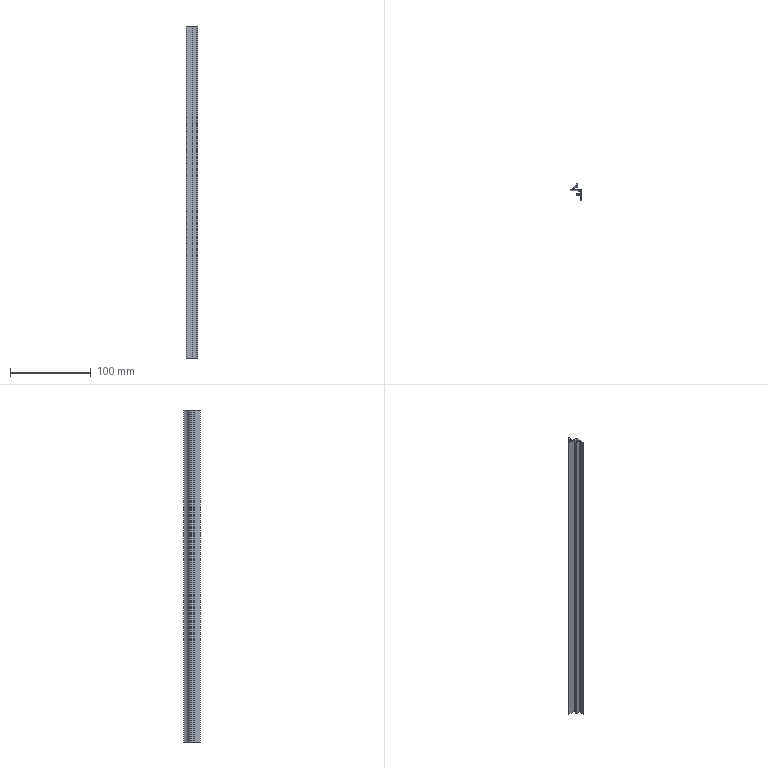Part | SolidWorks | features BaseBody 1, ICE 1, MoveFace 1 | 1 solid | 27 faces | box 14 x 20.3 x 410 mm | volume 20875 mm3 | plane 20 | cylinder 7 | commonest cylinder face diameters 0.387 x2 0.8 x2 0.4 x1 20 x1 22 x1
STEP:
#1=CARTESIAN_POINT('',(-5.304,-0.625,200.));
#2=VERTEX_POINT('',#1);
#3=CARTESIAN_POINT('',(-5.449,-0.8125,200.));
#4=VERTEX_POINT('',#3);
#5=CARTESIAN_POINT('',(-5.255,-0.8125,200.));
#6=DIRECTION('',(0.,0.,1.));
#7=DIRECTION('',(-1.,0.,0.));
#8=AXIS2_PLACEMENT_3D('',#5,#6,#7);
#9=CIRCLE('',#8,0.1937);
#10=EDGE_CURVE('',#2,#4,#9,.T.);
#11=ORIENTED_EDGE('',*,*,#10,.T.);
#12=CARTESIAN_POINT('',(-5.449,-0.8125,-210.));
#13=VERTEX_POINT('',#12);
#14=CARTESIAN_POINT('',(-5.449,-0.8125,230.));
#15=DIRECTION('',(0.,0.,-1.));
#16=VECTOR('',#15,1000.);
#17=LINE('',#14,#16);
#18=EDGE_CURVE('',#4,#13,#17,.T.);
#19=ORIENTED_EDGE('',*,*,#18,.T.);
#20=CARTESIAN_POINT('',(-5.304,-0.625,-210.));
#21=VERTEX_POINT('',#20);
#22=CARTESIAN_POINT('',(-5.255,-0.8125,-210.));
#23=DIRECTION('',(0.,0.,-1.));
#24=DIRECTION('',(1.,0.,0.));
#25=AXIS2_PLACEMENT_3D('',#22,#23,#24);
#26=CIRCLE('',#25,0.1937);
#27=EDGE_CURVE('',#13,#21,#26,.T.);
#28=ORIENTED_EDGE('',*,*,#27,.T.);
#29=CARTESIAN_POINT('',(-5.304,-0.625,230.));
#30=DIRECTION('',(0.,0.,-1.));
#31=VECTOR('',#30,1000.);
#32=LINE('',#29,#31);
#33=EDGE_CURVE('',#2,#21,#32,.T.);
#34=ORIENTED_EDGE('',*,*,#33,.F.);
#35=EDGE_LOOP('',(#11,#19,#28,#34));
#36=FACE_OUTER_BOUND('',#35,.T.);
#37=CARTESIAN_POINT('',(-5.255,-0.8125,230.));
#38=DIRECTION('',(0.,0.,-1.));
#39=DIRECTION('',(-1.,0.,0.));
#40=AXIS2_PLACEMENT_3D('',#37,#38,#39);
#41=CYLINDRICAL_SURFACE('',#40,0.1937);
#42=ADVANCED_FACE('',(#36),#41,.F.);
#43=CARTESIAN_POINT('',(5.,-1.,-210.));
#44=VERTEX_POINT('',#43);
#45=CARTESIAN_POINT('',(5.,-14.3,-210.));
#46=VERTEX_POINT('',#45);
#47=CARTESIAN_POINT('',(5.,29.623,-210.));
#48=DIRECTION('',(0.,-1.,0.));
#49=VECTOR('',#48,1000.);
#50=LINE('',#47,#49);
#51=EDGE_CURVE('',#44,#46,#50,.T.);
#52=ORIENTED_EDGE('',*,*,#51,.F.);
#53=CARTESIAN_POINT('',(5.,-1.,200.));
#54=VERTEX_POINT('',#53);
#55=CARTESIAN_POINT('',(5.,-1.,230.));
#56=DIRECTION('',(0.,0.,-1.));
#57=VECTOR('',#56,1000.);
#58=LINE('',#55,#57);
#59=EDGE_CURVE('',#54,#44,#58,.T.);
#60=ORIENTED_EDGE('',*,*,#59,.F.);
#61=CARTESIAN_POINT('',(5.,-14.3,200.));
#62=VERTEX_POINT('',#61);
#63=CARTESIAN_POINT('',(5.,-14.3,200.));
#64=DIRECTION('',(0.,1.,0.));
#65=VECTOR('',#64,1000.);
#66=LINE('',#63,#65);
#67=EDGE_CURVE('',#62,#54,#66,.T.);
#68=ORIENTED_EDGE('',*,*,#67,.F.);
#69=CARTESIAN_POINT('',(5.,-14.3,230.));
#70=DIRECTION('',(0.,0.,1.));
#71=VECTOR('',#70,1000.);
#72=LINE('',#69,#71);
#73=EDGE_CURVE('',#46,#62,#72,.T.);
#74=ORIENTED_EDGE('',*,*,#73,.F.);
#75=EDGE_LOOP('',(#52,#60,#68,#74));
#76=FACE_OUTER_BOUND('',#75,.T.);
#77=CARTESIAN_POINT('',(5.,-14.3,230.));
#78=DIRECTION('',(-1.,0.,0.));
#79=DIRECTION('',(0.,0.,1.));
#80=AXIS2_PLACEMENT_3D('',#77,#78,#79);
#81=PLANE('',#80);
#82=ADVANCED_FACE('',(#76),#81,.F.);
#83=CARTESIAN_POINT('',(-9.,-2.,-210.));
#84=VERTEX_POINT('',#83);
#85=CARTESIAN_POINT('',(-9.,-2.,200.));
#86=VERTEX_POINT('',#85);
#87=CARTESIAN_POINT('',(-9.,-2.,230.));
#88=DIRECTION('',(0.,0.,1.));
#89=VECTOR('',#88,1000.);
#90=LINE('',#87,#89);
#91=EDGE_CURVE('',#84,#86,#90,.T.);
#92=ORIENTED_EDGE('',*,*,#91,.F.);
#93=CARTESIAN_POINT('',(0.9,-2.,-210.));
#94=VERTEX_POINT('',#93);
#95=CARTESIAN_POINT('',(5.,-2.,-210.));
#96=DIRECTION('',(-1.,0.,0.));
#97=VECTOR('',#96,1000.);
#98=LINE('',#95,#97);
#99=EDGE_CURVE('',#94,#84,#98,.T.);
#100=ORIENTED_EDGE('',*,*,#99,.F.);
#101=CARTESIAN_POINT('',(0.9,-2.,200.));
#102=VERTEX_POINT('',#101);
#103=CARTESIAN_POINT('',(0.9,-2.,230.));
#104=DIRECTION('',(0.,0.,-1.));
#105=VECTOR('',#104,1000.);
#106=LINE('',#103,#105);
#107=EDGE_CURVE('',#102,#94,#106,.T.);
#108=ORIENTED_EDGE('',*,*,#107,.F.);
#109=CARTESIAN_POINT('',(5.,-2.,200.));
#110=DIRECTION('',(1.,0.,0.));
#111=VECTOR('',#110,1000.);
#112=LINE('',#109,#111);
#113=EDGE_CURVE('',#86,#102,#112,.T.);
#114=ORIENTED_EDGE('',*,*,#113,.F.);
#115=EDGE_LOOP('',(#92,#100,#108,#114));
#116=FACE_OUTER_BOUND('',#115,.T.);
#117=CARTESIAN_POINT('',(-9.,-2.,230.));
#118=DIRECTION('',(0.,1.,0.));
#119=DIRECTION('',(0.,0.,1.));
#120=AXIS2_PLACEMENT_3D('',#117,#118,#119);
#121=PLANE('',#120);
#122=ADVANCED_FACE('',(#116),#121,.F.);
#123=CARTESIAN_POINT('',(4.,-6.,200.));
#124=VERTEX_POINT('',#123);
#125=CARTESIAN_POINT('',(4.,-3.,200.));
#126=VERTEX_POINT('',#125);
#127=CARTESIAN_POINT('',(4.,29.623,200.));
#128=DIRECTION('',(0.,1.,0.));
#129=VECTOR('',#128,1000.);
#130=LINE('',#127,#129);
#131=EDGE_CURVE('',#124,#126,#130,.T.);
#132=ORIENTED_EDGE('',*,*,#131,.F.);
#133=CARTESIAN_POINT('',(1.,-6.,200.));
#134=VERTEX_POINT('',#133);
#135=CARTESIAN_POINT('',(5.,-6.,200.));
#136=DIRECTION('',(1.,0.,0.));
#137=VECTOR('',#136,1000.);
#138=LINE('',#135,#137);
#139=EDGE_CURVE('',#134,#124,#138,.T.);
#140=ORIENTED_EDGE('',*,*,#139,.F.);
#141=CARTESIAN_POINT('',(1.,-6.7,200.));
#142=VERTEX_POINT('',#141);
#143=CARTESIAN_POINT('',(1.,-6.,200.));
#144=DIRECTION('',(0.,-1.,0.));
#145=VECTOR('',#144,1000.);
#146=LINE('',#143,#145);
#147=EDGE_CURVE('',#134,#142,#146,.T.);
#148=ORIENTED_EDGE('',*,*,#147,.T.);
#149=CARTESIAN_POINT('',(-1.7,-6.7,200.));
#150=VERTEX_POINT('',#149);
#151=CARTESIAN_POINT('',(5.,-6.7,200.));
#152=DIRECTION('',(1.,0.,0.));
#153=VECTOR('',#152,1000.);
#154=LINE('',#151,#153);
#155=EDGE_CURVE('',#150,#142,#154,.T.);
#156=ORIENTED_EDGE('',*,*,#155,.F.);
#157=CARTESIAN_POINT('',(-1.7,-7.7,200.));
#158=VERTEX_POINT('',#157);
#159=CARTESIAN_POINT('',(-1.7,-6.7,200.));
#160=DIRECTION('',(0.,-1.,0.));
#161=VECTOR('',#160,1000.);
#162=LINE('',#159,#161);
#163=EDGE_CURVE('',#150,#158,#162,.T.);
#164=ORIENTED_EDGE('',*,*,#163,.T.);
#165=CARTESIAN_POINT('',(4.,-7.7,200.));
#166=VERTEX_POINT('',#165);
#167=CARTESIAN_POINT('',(5.,-7.7,200.));
#168=DIRECTION('',(-1.,0.,0.));
#169=VECTOR('',#168,1000.);
#170=LINE('',#167,#169);
#171=EDGE_CURVE('',#166,#158,#170,.T.);
#172=ORIENTED_EDGE('',*,*,#171,.F.);
#173=CARTESIAN_POINT('',(4.,-14.3,200.));
#174=VERTEX_POINT('',#173);
#175=CARTESIAN_POINT('',(4.,29.623,200.));
#176=DIRECTION('',(0.,1.,0.));
#177=VECTOR('',#176,1000.);
#178=LINE('',#175,#177);
#179=EDGE_CURVE('',#174,#166,#178,.T.);
#180=ORIENTED_EDGE('',*,*,#179,.F.);
#181=CARTESIAN_POINT('',(5.,-14.3,200.));
#182=DIRECTION('',(-1.,0.,0.));
#183=VECTOR('',#182,1000.);
#184=LINE('',#181,#183);
#185=EDGE_CURVE('',#62,#174,#184,.T.);
#186=ORIENTED_EDGE('',*,*,#185,.F.);
#187=ORIENTED_EDGE('',*,*,#67,.T.);
#188=CARTESIAN_POINT('',(-5.207,-1.,200.));
#189=VERTEX_POINT('',#188);
#190=CARTESIAN_POINT('',(5.,-1.,200.));
#191=DIRECTION('',(1.,0.,0.));
#192=VECTOR('',#191,1000.);
#193=LINE('',#190,#192);
#194=EDGE_CURVE('',#189,#54,#193,.T.);
#195=ORIENTED_EDGE('',*,*,#194,.F.);
#196=CARTESIAN_POINT('',(-5.255,-0.8125,200.));
#197=DIRECTION('',(0.,0.,1.));
#198=DIRECTION('',(-1.,0.,0.));
#199=AXIS2_PLACEMENT_3D('',#196,#197,#198);
#200=CIRCLE('',#199,0.1937);
#201=EDGE_CURVE('',#4,#189,#200,.T.);
#202=ORIENTED_EDGE('',*,*,#201,.F.);
#203=ORIENTED_EDGE('',*,*,#10,.F.);
#204=CARTESIAN_POINT('',(-1.368,3.063,200.));
#205=VERTEX_POINT('',#204);
#206=CARTESIAN_POINT('',(-10.628,9.,200.));
#207=DIRECTION('',(0.,0.,1.));
#208=DIRECTION('',(-1.,0.,0.));
#209=AXIS2_PLACEMENT_3D('',#206,#207,#208);
#210=CIRCLE('',#209,11.);
#211=EDGE_CURVE('',#2,#205,#210,.T.);
#212=ORIENTED_EDGE('',*,*,#211,.T.);
#213=CARTESIAN_POINT('',(-1.,2.955,200.));
#214=VERTEX_POINT('',#213);
#215=CARTESIAN_POINT('',(-1.2,2.955,200.));
#216=DIRECTION('',(0.,0.,1.));
#217=DIRECTION('',(-1.,0.,0.));
#218=AXIS2_PLACEMENT_3D('',#215,#216,#217);
#219=CIRCLE('',#218,0.2);
#220=EDGE_CURVE('',#214,#205,#219,.T.);
#221=ORIENTED_EDGE('',*,*,#220,.F.);
#222=CARTESIAN_POINT('',(-1.,1.5,200.));
#223=VERTEX_POINT('',#222);
#224=CARTESIAN_POINT('',(-1.,2.955,200.));
#225=DIRECTION('',(0.,1.,0.));
#226=VECTOR('',#225,1000.);
#227=LINE('',#224,#226);
#228=EDGE_CURVE('',#223,#214,#227,.T.);
#229=ORIENTED_EDGE('',*,*,#228,.F.);
#230=CARTESIAN_POINT('',(0.,1.5,200.));
#231=VERTEX_POINT('',#230);
#232=CARTESIAN_POINT('',(-1.,1.5,200.));
#233=DIRECTION('',(-1.,0.,0.));
#234=VECTOR('',#233,1000.);
#235=LINE('',#232,#234);
#236=EDGE_CURVE('',#231,#223,#235,.T.);
#237=ORIENTED_EDGE('',*,*,#236,.F.);
#238=CARTESIAN_POINT('',(0.,6.,200.));
#239=VERTEX_POINT('',#238);
#240=CARTESIAN_POINT('',(0.,1.5,200.));
#241=DIRECTION('',(0.,-1.,0.));
#242=VECTOR('',#241,1000.);
#243=LINE('',#240,#242);
#244=EDGE_CURVE('',#239,#231,#243,.T.);
#245=ORIENTED_EDGE('',*,*,#244,.F.);
#246=CARTESIAN_POINT('',(-0.8,6.,200.));
#247=VERTEX_POINT('',#246);
#248=CARTESIAN_POINT('',(0.,6.,200.));
#249=DIRECTION('',(1.,0.,0.));
#250=VECTOR('',#249,1000.);
#251=LINE('',#248,#250);
#252=EDGE_CURVE('',#247,#239,#251,.T.);
#253=ORIENTED_EDGE('',*,*,#252,.F.);
#254=CARTESIAN_POINT('',(-1.178,5.731,200.));
#255=VERTEX_POINT('',#254);
#256=CARTESIAN_POINT('',(-0.8,5.6,200.));
#257=DIRECTION('',(0.,0.,1.));
#258=DIRECTION('',(-1.,0.,0.));
#259=AXIS2_PLACEMENT_3D('',#256,#257,#258);
#260=CIRCLE('',#259,0.4);
#261=EDGE_CURVE('',#247,#255,#260,.T.);
#262=ORIENTED_EDGE('',*,*,#261,.T.);
#263=CARTESIAN_POINT('',(-8.678,-0.8077,200.));
#264=VERTEX_POINT('',#263);
#265=CARTESIAN_POINT('',(-10.628,9.,200.));
#266=DIRECTION('',(0.,0.,1.));
#267=DIRECTION('',(-1.,0.,0.));
#268=AXIS2_PLACEMENT_3D('',#265,#266,#267);
#269=CIRCLE('',#268,10.);
#270=EDGE_CURVE('',#264,#255,#269,.T.);
#271=ORIENTED_EDGE('',*,*,#270,.F.);
#272=CARTESIAN_POINT('',(-9.,-1.2,200.));
#273=VERTEX_POINT('',#272);
#274=CARTESIAN_POINT('',(-8.6,-1.2,200.));
#275=DIRECTION('',(0.,0.,1.));
#276=DIRECTION('',(-1.,0.,0.));
#277=AXIS2_PLACEMENT_3D('',#274,#275,#276);
#278=CIRCLE('',#277,0.4);
#279=EDGE_CURVE('',#264,#273,#278,.T.);
#280=ORIENTED_EDGE('',*,*,#279,.T.);
#281=CARTESIAN_POINT('',(-9.,8.,200.));
#282=DIRECTION('',(0.,-1.,0.));
#283=VECTOR('',#282,1000.);
#284=LINE('',#281,#283);
#285=EDGE_CURVE('',#273,#86,#284,.T.);
#286=ORIENTED_EDGE('',*,*,#285,.T.);
#287=ORIENTED_EDGE('',*,*,#113,.T.);
#288=CARTESIAN_POINT('',(0.9,-3.,200.));
#289=VERTEX_POINT('',#288);
#290=CARTESIAN_POINT('',(0.9,29.623,200.));
#291=DIRECTION('',(0.,1.,0.));
#292=VECTOR('',#291,1000.);
#293=LINE('',#290,#292);
#294=EDGE_CURVE('',#289,#102,#293,.T.);
#295=ORIENTED_EDGE('',*,*,#294,.F.);
#296=CARTESIAN_POINT('',(5.,-3.,200.));
#297=DIRECTION('',(-1.,0.,0.));
#298=VECTOR('',#297,1000.);
#299=LINE('',#296,#298);
#300=EDGE_CURVE('',#126,#289,#299,.T.);
#301=ORIENTED_EDGE('',*,*,#300,.F.);
#302=EDGE_LOOP('',(#132,#140,#148,#156,#164,#172,#180,#186,#187,#195,#202,#203,#212,#221,#229,#237,#245,#253,#262,#271,#280,#286,#287,#295,#301));
#303=FACE_OUTER_BOUND('',#302,.T.);
#304=CARTESIAN_POINT('',(5.,29.623,200.));
#305=DIRECTION('',(0.,0.,-1.));
#306=DIRECTION('',(-1.,0.,0.));
#307=AXIS2_PLACEMENT_3D('',#304,#305,#306);
#308=PLANE('',#307);
#309=ADVANCED_FACE('',(#303),#308,.F.);
#310=ORIENTED_EDGE('',*,*,#185,.T.);
#311=CARTESIAN_POINT('',(4.,-14.3,-210.));
#312=VERTEX_POINT('',#311);
#313=CARTESIAN_POINT('',(4.,-14.3,230.));
#314=DIRECTION('',(0.,0.,1.));
#315=VECTOR('',#314,1000.);
#316=LINE('',#313,#315);
#317=EDGE_CURVE('',#312,#174,#316,.T.);
#318=ORIENTED_EDGE('',*,*,#317,.F.);
#319=CARTESIAN_POINT('',(5.,-14.3,-210.));
#320=DIRECTION('',(-1.,0.,0.));
#321=VECTOR('',#320,1000.);
#322=LINE('',#319,#321);
#323=EDGE_CURVE('',#46,#312,#322,.T.);
#324=ORIENTED_EDGE('',*,*,#323,.F.);
#325=ORIENTED_EDGE('',*,*,#73,.T.);
#326=EDGE_LOOP('',(#310,#318,#324,#325));
#327=FACE_OUTER_BOUND('',#326,.T.);
#328=CARTESIAN_POINT('',(4.,-14.3,230.));
#329=DIRECTION('',(0.,1.,0.));
#330=DIRECTION('',(0.,0.,1.));
#331=AXIS2_PLACEMENT_3D('',#328,#329,#330);
#332=PLANE('',#331);
#333=ADVANCED_FACE('',(#327),#332,.F.);
#334=ORIENTED_EDGE('',*,*,#51,.T.);
#335=ORIENTED_EDGE('',*,*,#323,.T.);
#336=CARTESIAN_POINT('',(4.,-7.7,-210.));
#337=VERTEX_POINT('',#336);
#338=CARTESIAN_POINT('',(4.,-7.7,-210.));
#339=DIRECTION('',(0.,-1.,0.));
#340=VECTOR('',#339,1000.);
#341=LINE('',#338,#340);
#342=EDGE_CURVE('',#337,#312,#341,.T.);
#343=ORIENTED_EDGE('',*,*,#342,.F.);
#344=CARTESIAN_POINT('',(-1.7,-7.7,-210.));
#345=VERTEX_POINT('',#344);
#346=CARTESIAN_POINT('',(-1.7,-7.7,-210.));
#347=DIRECTION('',(1.,0.,0.));
#348=VECTOR('',#347,1000.);
#349=LINE('',#346,#348);
#350=EDGE_CURVE('',#345,#337,#349,.T.);
#351=ORIENTED_EDGE('',*,*,#350,.F.);
#352=CARTESIAN_POINT('',(-1.7,-6.7,-210.));
#353=VERTEX_POINT('',#352);
#354=CARTESIAN_POINT('',(-1.7,29.623,-210.));
#355=DIRECTION('',(0.,1.,0.));
#356=VECTOR('',#355,1000.);
#357=LINE('',#354,#356);
#358=EDGE_CURVE('',#345,#353,#357,.T.);
#359=ORIENTED_EDGE('',*,*,#358,.T.);
#360=CARTESIAN_POINT('',(1.,-6.7,-210.));
#361=VERTEX_POINT('',#360);
#362=CARTESIAN_POINT('',(1.,-6.7,-210.));
#363=DIRECTION('',(-1.,0.,0.));
#364=VECTOR('',#363,1000.);
#365=LINE('',#362,#364);
#366=EDGE_CURVE('',#361,#353,#365,.T.);
#367=ORIENTED_EDGE('',*,*,#366,.F.);
#368=CARTESIAN_POINT('',(1.,-6.,-210.));
#369=VERTEX_POINT('',#368);
#370=CARTESIAN_POINT('',(1.,29.623,-210.));
#371=DIRECTION('',(0.,1.,0.));
#372=VECTOR('',#371,1000.);
#373=LINE('',#370,#372);
#374=EDGE_CURVE('',#361,#369,#373,.T.);
#375=ORIENTED_EDGE('',*,*,#374,.T.);
#376=CARTESIAN_POINT('',(4.,-6.,-210.));
#377=VERTEX_POINT('',#376);
#378=CARTESIAN_POINT('',(4.,-6.,-210.));
#379=DIRECTION('',(-1.,0.,0.));
#380=VECTOR('',#379,1000.);
#381=LINE('',#378,#380);
#382=EDGE_CURVE('',#377,#369,#381,.T.);
#383=ORIENTED_EDGE('',*,*,#382,.F.);
#384=CARTESIAN_POINT('',(4.,-3.,-210.));
#385=VERTEX_POINT('',#384);
#386=CARTESIAN_POINT('',(4.,-3.,-210.));
#387=DIRECTION('',(0.,-1.,0.));
#388=VECTOR('',#387,1000.);
#389=LINE('',#386,#388);
#390=EDGE_CURVE('',#385,#377,#389,.T.);
#391=ORIENTED_EDGE('',*,*,#390,.F.);
#392=CARTESIAN_POINT('',(0.9,-3.,-210.));
#393=VERTEX_POINT('',#392);
#394=CARTESIAN_POINT('',(0.9,-3.,-210.));
#395=DIRECTION('',(1.,0.,0.));
#396=VECTOR('',#395,1000.);
#397=LINE('',#394,#396);
#398=EDGE_CURVE('',#393,#385,#397,.T.);
#399=ORIENTED_EDGE('',*,*,#398,.F.);
#400=CARTESIAN_POINT('',(0.9,-2.,-210.));
#401=DIRECTION('',(0.,-1.,0.));
#402=VECTOR('',#401,1000.);
#403=LINE('',#400,#402);
#404=EDGE_CURVE('',#94,#393,#403,.T.);
#405=ORIENTED_EDGE('',*,*,#404,.F.);
#406=ORIENTED_EDGE('',*,*,#99,.T.);
#407=CARTESIAN_POINT('',(-9.,-1.2,-210.));
#408=VERTEX_POINT('',#407);
#409=CARTESIAN_POINT('',(-9.,-1.2,-210.));
#410=DIRECTION('',(0.,-1.,0.));
#411=VECTOR('',#410,1000.);
#412=LINE('',#409,#411);
#413=EDGE_CURVE('',#408,#84,#412,.T.);
#414=ORIENTED_EDGE('',*,*,#413,.F.);
#415=CARTESIAN_POINT('',(-8.678,-0.8077,-210.));
#416=VERTEX_POINT('',#415);
#417=CARTESIAN_POINT('',(-8.6,-1.2,-210.));
#418=DIRECTION('',(0.,0.,-1.));
#419=DIRECTION('',(1.,0.,0.));
#420=AXIS2_PLACEMENT_3D('',#417,#418,#419);
#421=CIRCLE('',#420,0.4);
#422=EDGE_CURVE('',#408,#416,#421,.T.);
#423=ORIENTED_EDGE('',*,*,#422,.T.);
#424=CARTESIAN_POINT('',(-1.178,5.731,-210.));
#425=VERTEX_POINT('',#424);
#426=CARTESIAN_POINT('',(-10.628,9.,-210.));
#427=DIRECTION('',(0.,0.,-1.));
#428=DIRECTION('',(1.,0.,0.));
#429=AXIS2_PLACEMENT_3D('',#426,#427,#428);
#430=CIRCLE('',#429,10.);
#431=EDGE_CURVE('',#425,#416,#430,.T.);
#432=ORIENTED_EDGE('',*,*,#431,.F.);
#433=CARTESIAN_POINT('',(-0.8,6.,-210.));
#434=VERTEX_POINT('',#433);
#435=CARTESIAN_POINT('',(-0.8,5.6,-210.));
#436=DIRECTION('',(0.,0.,-1.));
#437=DIRECTION('',(1.,0.,0.));
#438=AXIS2_PLACEMENT_3D('',#435,#436,#437);
#439=CIRCLE('',#438,0.4);
#440=EDGE_CURVE('',#425,#434,#439,.T.);
#441=ORIENTED_EDGE('',*,*,#440,.T.);
#442=CARTESIAN_POINT('',(0.,6.,-210.));
#443=VERTEX_POINT('',#442);
#444=CARTESIAN_POINT('',(0.,6.,-210.));
#445=DIRECTION('',(-1.,0.,0.));
#446=VECTOR('',#445,1000.);
#447=LINE('',#444,#446);
#448=EDGE_CURVE('',#443,#434,#447,.T.);
#449=ORIENTED_EDGE('',*,*,#448,.F.);
#450=CARTESIAN_POINT('',(0.,1.5,-210.));
#451=VERTEX_POINT('',#450);
#452=CARTESIAN_POINT('',(0.,1.5,-210.));
#453=DIRECTION('',(0.,1.,0.));
#454=VECTOR('',#453,1000.);
#455=LINE('',#452,#454);
#456=EDGE_CURVE('',#451,#443,#455,.T.);
#457=ORIENTED_EDGE('',*,*,#456,.F.);
#458=CARTESIAN_POINT('',(-1.,1.5,-210.));
#459=VERTEX_POINT('',#458);
#460=CARTESIAN_POINT('',(-1.,1.5,-210.));
#461=DIRECTION('',(1.,0.,0.));
#462=VECTOR('',#461,1000.);
#463=LINE('',#460,#462);
#464=EDGE_CURVE('',#459,#451,#463,.T.);
#465=ORIENTED_EDGE('',*,*,#464,.F.);
#466=CARTESIAN_POINT('',(-1.,2.955,-210.));
#467=VERTEX_POINT('',#466);
#468=CARTESIAN_POINT('',(-1.,2.955,-210.));
#469=DIRECTION('',(0.,-1.,0.));
#470=VECTOR('',#469,1000.);
#471=LINE('',#468,#470);
#472=EDGE_CURVE('',#467,#459,#471,.T.);
#473=ORIENTED_EDGE('',*,*,#472,.F.);
#474=CARTESIAN_POINT('',(-1.368,3.063,-210.));
#475=VERTEX_POINT('',#474);
#476=CARTESIAN_POINT('',(-1.2,2.955,-210.));
#477=DIRECTION('',(0.,0.,-1.));
#478=DIRECTION('',(1.,0.,0.));
#479=AXIS2_PLACEMENT_3D('',#476,#477,#478);
#480=CIRCLE('',#479,0.2);
#481=EDGE_CURVE('',#475,#467,#480,.T.);
#482=ORIENTED_EDGE('',*,*,#481,.F.);
#483=CARTESIAN_POINT('',(-10.628,9.,-210.));
#484=DIRECTION('',(0.,0.,-1.));
#485=DIRECTION('',(1.,0.,0.));
#486=AXIS2_PLACEMENT_3D('',#483,#484,#485);
#487=CIRCLE('',#486,11.);
#488=EDGE_CURVE('',#475,#21,#487,.T.);
#489=ORIENTED_EDGE('',*,*,#488,.T.);
#490=ORIENTED_EDGE('',*,*,#27,.F.);
#491=CARTESIAN_POINT('',(-5.207,-1.,-210.));
#492=VERTEX_POINT('',#491);
#493=CARTESIAN_POINT('',(-5.255,-0.8125,-210.));
#494=DIRECTION('',(0.,0.,-1.));
#495=DIRECTION('',(1.,0.,0.));
#496=AXIS2_PLACEMENT_3D('',#493,#494,#495);
#497=CIRCLE('',#496,0.1937);
#498=EDGE_CURVE('',#492,#13,#497,.T.);
#499=ORIENTED_EDGE('',*,*,#498,.F.);
#500=CARTESIAN_POINT('',(5.,-1.,-210.));
#501=DIRECTION('',(-1.,0.,0.));
#502=VECTOR('',#501,1000.);
#503=LINE('',#500,#502);
#504=EDGE_CURVE('',#44,#492,#503,.T.);
#505=ORIENTED_EDGE('',*,*,#504,.F.);
#506=EDGE_LOOP('',(#334,#335,#343,#351,#359,#367,#375,#383,#391,#399,#405,#406,#414,#423,#432,#441,#449,#457,#465,#473,#482,#489,#490,#499,#505));
#507=FACE_OUTER_BOUND('',#506,.T.);
#508=CARTESIAN_POINT('',(5.,29.623,-210.));
#509=DIRECTION('',(0.,0.,1.));
#510=DIRECTION('',(1.,0.,0.));
#511=AXIS2_PLACEMENT_3D('',#508,#509,#510);
#512=PLANE('',#511);
#513=ADVANCED_FACE('',(#507),#512,.F.);
#514=ORIENTED_EDGE('',*,*,#59,.T.);
#515=ORIENTED_EDGE('',*,*,#504,.T.);
#516=CARTESIAN_POINT('',(-5.207,-1.,230.));
#517=DIRECTION('',(0.,0.,-1.));
#518=VECTOR('',#517,1000.);
#519=LINE('',#516,#518);
#520=EDGE_CURVE('',#189,#492,#519,.T.);
#521=ORIENTED_EDGE('',*,*,#520,.F.);
#522=ORIENTED_EDGE('',*,*,#194,.T.);
#523=EDGE_LOOP('',(#514,#515,#521,#522));
#524=FACE_OUTER_BOUND('',#523,.T.);
#525=CARTESIAN_POINT('',(5.,-1.,230.));
#526=DIRECTION('',(0.,-1.,0.));
#527=DIRECTION('',(0.,0.,-1.));
#528=AXIS2_PLACEMENT_3D('',#525,#526,#527);
#529=PLANE('',#528);
#530=ADVANCED_FACE('',(#524),#529,.F.);
#531=CARTESIAN_POINT('',(-9.,-1.2,230.));
#532=DIRECTION('',(0.,0.,1.));
#533=VECTOR('',#532,1000.);
#534=LINE('',#531,#533);
#535=EDGE_CURVE('',#408,#273,#534,.T.);
#536=ORIENTED_EDGE('',*,*,#535,.F.);
#537=ORIENTED_EDGE('',*,*,#413,.T.);
#538=ORIENTED_EDGE('',*,*,#91,.T.);
#539=ORIENTED_EDGE('',*,*,#285,.F.);
#540=EDGE_LOOP('',(#536,#537,#538,#539));
#541=FACE_OUTER_BOUND('',#540,.T.);
#542=CARTESIAN_POINT('',(-9.,-1.2,230.));
#543=DIRECTION('',(1.,0.,0.));
#544=DIRECTION('',(0.,0.,-1.));
#545=AXIS2_PLACEMENT_3D('',#542,#543,#544);
#546=PLANE('',#545);
#547=ADVANCED_FACE('',(#541),#546,.F.);
#548=ORIENTED_EDGE('',*,*,#294,.T.);
#549=ORIENTED_EDGE('',*,*,#107,.T.);
#550=ORIENTED_EDGE('',*,*,#404,.T.);
#551=CARTESIAN_POINT('',(0.9,-3.,230.));
#552=DIRECTION('',(0.,0.,-1.));
#553=VECTOR('',#552,1000.);
#554=LINE('',#551,#553);
#555=EDGE_CURVE('',#289,#393,#554,.T.);
#556=ORIENTED_EDGE('',*,*,#555,.F.);
#557=EDGE_LOOP('',(#548,#549,#550,#556));
#558=FACE_OUTER_BOUND('',#557,.T.);
#559=CARTESIAN_POINT('',(0.9,-2.,230.));
#560=DIRECTION('',(1.,0.,0.));
#561=DIRECTION('',(0.,0.,-1.));
#562=AXIS2_PLACEMENT_3D('',#559,#560,#561);
#563=PLANE('',#562);
#564=ADVANCED_FACE('',(#558),#563,.F.);
#565=ORIENTED_EDGE('',*,*,#300,.T.);
#566=ORIENTED_EDGE('',*,*,#555,.T.);
#567=ORIENTED_EDGE('',*,*,#398,.T.);
#568=CARTESIAN_POINT('',(4.,-3.,230.));
#569=DIRECTION('',(0.,0.,-1.));
#570=VECTOR('',#569,1000.);
#571=LINE('',#568,#570);
#572=EDGE_CURVE('',#126,#385,#571,.T.);
#573=ORIENTED_EDGE('',*,*,#572,.F.);
#574=EDGE_LOOP('',(#565,#566,#567,#573));
#575=FACE_OUTER_BOUND('',#574,.T.);
#576=CARTESIAN_POINT('',(0.9,-3.,230.));
#577=DIRECTION('',(0.,1.,0.));
#578=DIRECTION('',(0.,0.,1.));
#579=AXIS2_PLACEMENT_3D('',#576,#577,#578);
#580=PLANE('',#579);
#581=ADVANCED_FACE('',(#575),#580,.F.);
#582=ORIENTED_EDGE('',*,*,#131,.T.);
#583=ORIENTED_EDGE('',*,*,#572,.T.);
#584=ORIENTED_EDGE('',*,*,#390,.T.);
#585=CARTESIAN_POINT('',(4.,-6.,230.));
#586=DIRECTION('',(0.,0.,-1.));
#587=VECTOR('',#586,1000.);
#588=LINE('',#585,#587);
#589=EDGE_CURVE('',#124,#377,#588,.T.);
#590=ORIENTED_EDGE('',*,*,#589,.F.);
#591=EDGE_LOOP('',(#582,#583,#584,#590));
#592=FACE_OUTER_BOUND('',#591,.T.);
#593=CARTESIAN_POINT('',(4.,-3.,230.));
#594=DIRECTION('',(1.,0.,0.));
#595=DIRECTION('',(0.,0.,-1.));
#596=AXIS2_PLACEMENT_3D('',#593,#594,#595);
#597=PLANE('',#596);
#598=ADVANCED_FACE('',(#592),#597,.F.);
#599=ORIENTED_EDGE('',*,*,#139,.T.);
#600=ORIENTED_EDGE('',*,*,#589,.T.);
#601=ORIENTED_EDGE('',*,*,#382,.T.);
#602=CARTESIAN_POINT('',(1.,-6.,230.));
#603=DIRECTION('',(0.,0.,-1.));
#604=VECTOR('',#603,1000.);
#605=LINE('',#602,#604);
#606=EDGE_CURVE('',#134,#369,#605,.T.);
#607=ORIENTED_EDGE('',*,*,#606,.F.);
#608=EDGE_LOOP('',(#599,#600,#601,#607));
#609=FACE_OUTER_BOUND('',#608,.T.);
#610=CARTESIAN_POINT('',(4.,-6.,230.));
#611=DIRECTION('',(0.,-1.,0.));
#612=DIRECTION('',(0.,0.,-1.));
#613=AXIS2_PLACEMENT_3D('',#610,#611,#612);
#614=PLANE('',#613);
#615=ADVANCED_FACE('',(#609),#614,.F.);
#616=ORIENTED_EDGE('',*,*,#155,.T.);
#617=CARTESIAN_POINT('',(1.,-6.7,230.));
#618=DIRECTION('',(0.,0.,1.));
#619=VECTOR('',#618,1000.);
#620=LINE('',#617,#619);
#621=EDGE_CURVE('',#361,#142,#620,.T.);
#622=ORIENTED_EDGE('',*,*,#621,.F.);
#623=ORIENTED_EDGE('',*,*,#366,.T.);
#624=CARTESIAN_POINT('',(-1.7,-6.7,230.));
#625=DIRECTION('',(0.,0.,-1.));
#626=VECTOR('',#625,1000.);
#627=LINE('',#624,#626);
#628=EDGE_CURVE('',#150,#353,#627,.T.);
#629=ORIENTED_EDGE('',*,*,#628,.F.);
#630=EDGE_LOOP('',(#616,#622,#623,#629));
#631=FACE_OUTER_BOUND('',#630,.T.);
#632=CARTESIAN_POINT('',(1.,-6.7,230.));
#633=DIRECTION('',(0.,-1.,0.));
#634=DIRECTION('',(0.,0.,-1.));
#635=AXIS2_PLACEMENT_3D('',#632,#633,#634);
#636=PLANE('',#635);
#637=ADVANCED_FACE('',(#631),#636,.F.);
#638=ORIENTED_EDGE('',*,*,#171,.T.);
#639=CARTESIAN_POINT('',(-1.7,-7.7,230.));
#640=DIRECTION('',(0.,0.,1.));
#641=VECTOR('',#640,1000.);
#642=LINE('',#639,#641);
#643=EDGE_CURVE('',#345,#158,#642,.T.);
#644=ORIENTED_EDGE('',*,*,#643,.F.);
#645=ORIENTED_EDGE('',*,*,#350,.T.);
#646=CARTESIAN_POINT('',(4.,-7.7,230.));
#647=DIRECTION('',(0.,0.,-1.));
#648=VECTOR('',#647,1000.);
#649=LINE('',#646,#648);
#650=EDGE_CURVE('',#166,#337,#649,.T.);
#651=ORIENTED_EDGE('',*,*,#650,.F.);
#652=EDGE_LOOP('',(#638,#644,#645,#651));
#653=FACE_OUTER_BOUND('',#652,.T.);
#654=CARTESIAN_POINT('',(-1.7,-7.7,230.));
#655=DIRECTION('',(0.,1.,0.));
#656=DIRECTION('',(0.,0.,1.));
#657=AXIS2_PLACEMENT_3D('',#654,#655,#656);
#658=PLANE('',#657);
#659=ADVANCED_FACE('',(#653),#658,.F.);
#660=ORIENTED_EDGE('',*,*,#179,.T.);
#661=ORIENTED_EDGE('',*,*,#650,.T.);
#662=ORIENTED_EDGE('',*,*,#342,.T.);
#663=ORIENTED_EDGE('',*,*,#317,.T.);
#664=EDGE_LOOP('',(#660,#661,#662,#663));
#665=FACE_OUTER_BOUND('',#664,.T.);
#666=CARTESIAN_POINT('',(4.,-7.7,230.));
#667=DIRECTION('',(1.,0.,0.));
#668=DIRECTION('',(0.,0.,-1.));
#669=AXIS2_PLACEMENT_3D('',#666,#667,#668);
#670=PLANE('',#669);
#671=ADVANCED_FACE('',(#665),#670,.F.);
#672=ORIENTED_EDGE('',*,*,#18,.F.);
#673=ORIENTED_EDGE('',*,*,#201,.T.);
#674=ORIENTED_EDGE('',*,*,#520,.T.);
#675=ORIENTED_EDGE('',*,*,#498,.T.);
#676=EDGE_LOOP('',(#672,#673,#674,#675));
#677=FACE_OUTER_BOUND('',#676,.T.);
#678=CARTESIAN_POINT('',(-5.255,-0.8125,230.));
#679=DIRECTION('',(0.,0.,-1.));
#680=DIRECTION('',(-1.,0.,0.));
#681=AXIS2_PLACEMENT_3D('',#678,#679,#680);
#682=CYLINDRICAL_SURFACE('',#681,0.1937);
#683=ADVANCED_FACE('',(#677),#682,.F.);
#684=CARTESIAN_POINT('',(-1.,2.955,230.));
#685=DIRECTION('',(0.,0.,1.));
#686=VECTOR('',#685,1000.);
#687=LINE('',#684,#686);
#688=EDGE_CURVE('',#467,#214,#687,.T.);
#689=ORIENTED_EDGE('',*,*,#688,.F.);
#690=ORIENTED_EDGE('',*,*,#472,.T.);
#691=CARTESIAN_POINT('',(-1.,1.5,230.));
#692=DIRECTION('',(0.,0.,-1.));
#693=VECTOR('',#692,1000.);
#694=LINE('',#691,#693);
#695=EDGE_CURVE('',#223,#459,#694,.T.);
#696=ORIENTED_EDGE('',*,*,#695,.F.);
#697=ORIENTED_EDGE('',*,*,#228,.T.);
#698=EDGE_LOOP('',(#689,#690,#696,#697));
#699=FACE_OUTER_BOUND('',#698,.T.);
#700=CARTESIAN_POINT('',(-1.,2.955,230.));
#701=DIRECTION('',(1.,0.,0.));
#702=DIRECTION('',(0.,0.,-1.));
#703=AXIS2_PLACEMENT_3D('',#700,#701,#702);
#704=PLANE('',#703);
#705=ADVANCED_FACE('',(#699),#704,.F.);
#706=ORIENTED_EDGE('',*,*,#488,.F.);
#707=CARTESIAN_POINT('',(-1.368,3.063,230.));
#708=DIRECTION('',(0.,0.,1.));
#709=VECTOR('',#708,1000.);
#710=LINE('',#707,#709);
#711=EDGE_CURVE('',#475,#205,#710,.T.);
#712=ORIENTED_EDGE('',*,*,#711,.T.);
#713=ORIENTED_EDGE('',*,*,#211,.F.);
#714=ORIENTED_EDGE('',*,*,#33,.T.);
#715=EDGE_LOOP('',(#706,#712,#713,#714));
#716=FACE_OUTER_BOUND('',#715,.T.);
#717=CARTESIAN_POINT('',(-10.628,9.,230.));
#718=DIRECTION('',(0.,0.,-1.));
#719=DIRECTION('',(-1.,0.,0.));
#720=AXIS2_PLACEMENT_3D('',#717,#718,#719);
#721=CYLINDRICAL_SURFACE('',#720,11.);
#722=ADVANCED_FACE('',(#716),#721,.T.);
#723=CARTESIAN_POINT('',(-1.178,5.731,230.));
#724=DIRECTION('',(0.,0.,1.));
#725=VECTOR('',#724,1000.);
#726=LINE('',#723,#725);
#727=EDGE_CURVE('',#425,#255,#726,.T.);
#728=ORIENTED_EDGE('',*,*,#727,.F.);
#729=ORIENTED_EDGE('',*,*,#431,.T.);
#730=CARTESIAN_POINT('',(-8.678,-0.8077,230.));
#731=DIRECTION('',(0.,0.,-1.));
#732=VECTOR('',#731,1000.);
#733=LINE('',#730,#732);
#734=EDGE_CURVE('',#264,#416,#733,.T.);
#735=ORIENTED_EDGE('',*,*,#734,.F.);
#736=ORIENTED_EDGE('',*,*,#270,.T.);
#737=EDGE_LOOP('',(#728,#729,#735,#736));
#738=FACE_OUTER_BOUND('',#737,.T.);
#739=CARTESIAN_POINT('',(-10.628,9.,230.));
#740=DIRECTION('',(0.,0.,-1.));
#741=DIRECTION('',(-1.,0.,0.));
#742=AXIS2_PLACEMENT_3D('',#739,#740,#741);
#743=CYLINDRICAL_SURFACE('',#742,10.);
#744=ADVANCED_FACE('',(#738),#743,.F.);
#745=CARTESIAN_POINT('',(0.,1.5,230.));
#746=DIRECTION('',(0.,0.,1.));
#747=VECTOR('',#746,1000.);
#748=LINE('',#745,#747);
#749=EDGE_CURVE('',#451,#231,#748,.T.);
#750=ORIENTED_EDGE('',*,*,#749,.F.);
#751=ORIENTED_EDGE('',*,*,#456,.T.);
#752=CARTESIAN_POINT('',(0.,6.,230.));
#753=DIRECTION('',(0.,0.,-1.));
#754=VECTOR('',#753,1000.);
#755=LINE('',#752,#754);
#756=EDGE_CURVE('',#239,#443,#755,.T.);
#757=ORIENTED_EDGE('',*,*,#756,.F.);
#758=ORIENTED_EDGE('',*,*,#244,.T.);
#759=EDGE_LOOP('',(#750,#751,#757,#758));
#760=FACE_OUTER_BOUND('',#759,.T.);
#761=CARTESIAN_POINT('',(0.,1.5,230.));
#762=DIRECTION('',(-1.,0.,0.));
#763=DIRECTION('',(0.,0.,1.));
#764=AXIS2_PLACEMENT_3D('',#761,#762,#763);
#765=PLANE('',#764);
#766=ADVANCED_FACE('',(#760),#765,.F.);
#767=ORIENTED_EDGE('',*,*,#422,.F.);
#768=ORIENTED_EDGE('',*,*,#535,.T.);
#769=ORIENTED_EDGE('',*,*,#279,.F.);
#770=ORIENTED_EDGE('',*,*,#734,.T.);
#771=EDGE_LOOP('',(#767,#768,#769,#770));
#772=FACE_OUTER_BOUND('',#771,.T.);
#773=CARTESIAN_POINT('',(-8.6,-1.2,230.));
#774=DIRECTION('',(0.,0.,-1.));
#775=DIRECTION('',(-1.,0.,0.));
#776=AXIS2_PLACEMENT_3D('',#773,#774,#775);
#777=CYLINDRICAL_SURFACE('',#776,0.4);
#778=ADVANCED_FACE('',(#772),#777,.T.);
#779=ORIENTED_EDGE('',*,*,#147,.F.);
#780=ORIENTED_EDGE('',*,*,#606,.T.);
#781=ORIENTED_EDGE('',*,*,#374,.F.);
#782=ORIENTED_EDGE('',*,*,#621,.T.);
#783=EDGE_LOOP('',(#779,#780,#781,#782));
#784=FACE_OUTER_BOUND('',#783,.T.);
#785=CARTESIAN_POINT('',(1.,-6.,230.));
#786=DIRECTION('',(1.,0.,0.));
#787=DIRECTION('',(0.,0.,-1.));
#788=AXIS2_PLACEMENT_3D('',#785,#786,#787);
#789=PLANE('',#788);
#790=ADVANCED_FACE('',(#784),#789,.F.);
#791=ORIENTED_EDGE('',*,*,#163,.F.);
#792=ORIENTED_EDGE('',*,*,#628,.T.);
#793=ORIENTED_EDGE('',*,*,#358,.F.);
#794=ORIENTED_EDGE('',*,*,#643,.T.);
#795=EDGE_LOOP('',(#791,#792,#793,#794));
#796=FACE_OUTER_BOUND('',#795,.T.);
#797=CARTESIAN_POINT('',(-1.7,-6.7,230.));
#798=DIRECTION('',(1.,0.,0.));
#799=DIRECTION('',(0.,0.,-1.));
#800=AXIS2_PLACEMENT_3D('',#797,#798,#799);
#801=PLANE('',#800);
#802=ADVANCED_FACE('',(#796),#801,.F.);
#803=ORIENTED_EDGE('',*,*,#711,.F.);
#804=ORIENTED_EDGE('',*,*,#481,.T.);
#805=ORIENTED_EDGE('',*,*,#688,.T.);
#806=ORIENTED_EDGE('',*,*,#220,.T.);
#807=EDGE_LOOP('',(#803,#804,#805,#806));
#808=FACE_OUTER_BOUND('',#807,.T.);
#809=CARTESIAN_POINT('',(-1.2,2.955,230.));
#810=DIRECTION('',(0.,0.,-1.));
#811=DIRECTION('',(-1.,0.,0.));
#812=AXIS2_PLACEMENT_3D('',#809,#810,#811);
#813=CYLINDRICAL_SURFACE('',#812,0.2);
#814=ADVANCED_FACE('',(#808),#813,.F.);
#815=ORIENTED_EDGE('',*,*,#695,.T.);
#816=ORIENTED_EDGE('',*,*,#464,.T.);
#817=ORIENTED_EDGE('',*,*,#749,.T.);
#818=ORIENTED_EDGE('',*,*,#236,.T.);
#819=EDGE_LOOP('',(#815,#816,#817,#818));
#820=FACE_OUTER_BOUND('',#819,.T.);
#821=CARTESIAN_POINT('',(-1.,1.5,230.));
#822=DIRECTION('',(0.,1.,0.));
#823=DIRECTION('',(0.,0.,1.));
#824=AXIS2_PLACEMENT_3D('',#821,#822,#823);
#825=PLANE('',#824);
#826=ADVANCED_FACE('',(#820),#825,.F.);
#827=ORIENTED_EDGE('',*,*,#440,.F.);
#828=ORIENTED_EDGE('',*,*,#727,.T.);
#829=ORIENTED_EDGE('',*,*,#261,.F.);
#830=CARTESIAN_POINT('',(-0.8,6.,230.));
#831=DIRECTION('',(0.,0.,-1.));
#832=VECTOR('',#831,1000.);
#833=LINE('',#830,#832);
#834=EDGE_CURVE('',#247,#434,#833,.T.);
#835=ORIENTED_EDGE('',*,*,#834,.T.);
#836=EDGE_LOOP('',(#827,#828,#829,#835));
#837=FACE_OUTER_BOUND('',#836,.T.);
#838=CARTESIAN_POINT('',(-0.8,5.6,230.));
#839=DIRECTION('',(0.,0.,-1.));
#840=DIRECTION('',(-1.,0.,0.));
#841=AXIS2_PLACEMENT_3D('',#838,#839,#840);
#842=CYLINDRICAL_SURFACE('',#841,0.4);
#843=ADVANCED_FACE('',(#837),#842,.T.);
#844=ORIENTED_EDGE('',*,*,#756,.T.);
#845=ORIENTED_EDGE('',*,*,#448,.T.);
#846=ORIENTED_EDGE('',*,*,#834,.F.);
#847=ORIENTED_EDGE('',*,*,#252,.T.);
#848=EDGE_LOOP('',(#844,#845,#846,#847));
#849=FACE_OUTER_BOUND('',#848,.T.);
#850=CARTESIAN_POINT('',(0.,6.,230.));
#851=DIRECTION('',(0.,-1.,0.));
#852=DIRECTION('',(0.,0.,-1.));
#853=AXIS2_PLACEMENT_3D('',#850,#851,#852);
#854=PLANE('',#853);
#855=ADVANCED_FACE('',(#849),#854,.F.);
#856=CLOSED_SHELL('',(#42,#82,#122,#309,#333,#513,#530,#547,#564,#581,#598,#615,#637,#659,#671,#683,#705,#722,#744,#766,#778,#790,#802,#814,#826,#843,#855));
#857=MANIFOLD_SOLID_BREP('',#856);
#858=CARTESIAN_POINT('',(0.,0.,0.));
#859=DIRECTION('',(0.,0.,1.));
#860=DIRECTION('',(1.,0.,0.));
#861=AXIS2_PLACEMENT_3D('',#858,#859,#860);
#862=(LENGTH_UNIT()NAMED_UNIT(*)SI_UNIT(.MILLI.,.METRE.));
#863=UNCERTAINTY_MEASURE_WITH_UNIT(LENGTH_MEASURE(0.00001),#862,'','');
#864=(NAMED_UNIT(*)PLANE_ANGLE_UNIT()SI_UNIT($,.RADIAN.));
#865=(NAMED_UNIT(*)SI_UNIT($,.STERADIAN.)SOLID_ANGLE_UNIT());
#866=(GEOMETRIC_REPRESENTATION_CONTEXT(3)GLOBAL_UNCERTAINTY_ASSIGNED_CONTEXT((#863))GLOBAL_UNIT_ASSIGNED_CONTEXT((#862,#864,#865))REPRESENTATION_CONTEXT('',''));
#867=ADVANCED_BREP_SHAPE_REPRESENTATION('',(#857,#861),#866);